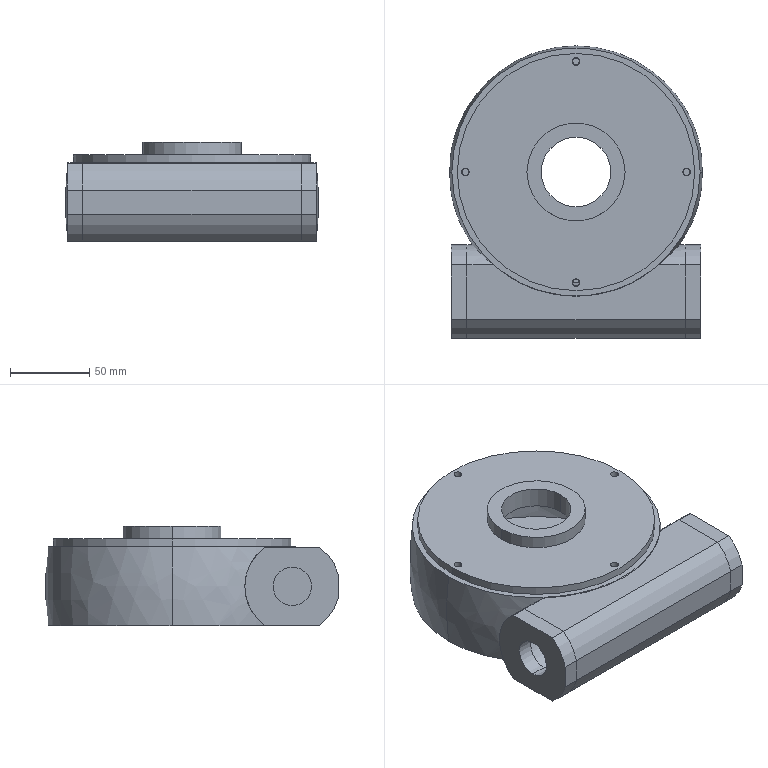Part | SolidWorks | features BaseBody 4 | 4 solids | 107 faces | box 160 x 184.969 x 63 mm | volume 414502 mm3 | cylinder 64 | plane 22 | cone 16 | spline 5 | commonest cylinder face diameters 4.2 x32 60 x10 5 x8 24.22 x2 42 x2 44 x2